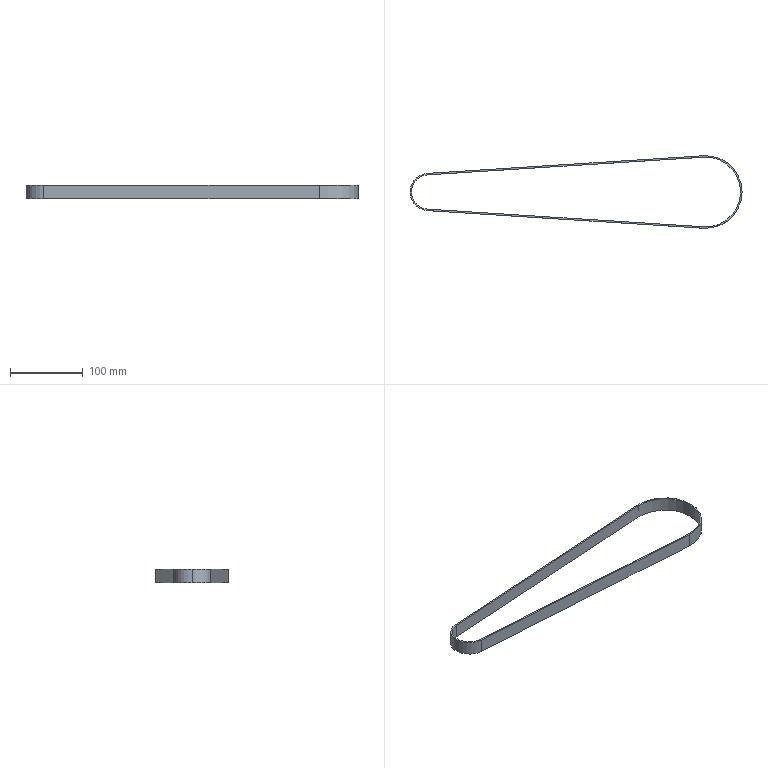Part | STEP file | Timing belt_3 | 1 solid | 12 faces | box 455.684 x 99.713 x 19.05 mm | volume 38426 mm3 | cylinder 6 | plane 6 | commonest cylinder face diameters 47.139 x2 51.203 x2 95.649 x1 99.713 x1
STEP:
#1=CARTESIAN_POINT('',(0.,0.,0.));
#2=DIRECTION('',(0.,0.,1.));
#3=DIRECTION('',(1.,0.,0.));
#4=AXIS2_PLACEMENT_3D('',#1,#2,#3);
#5=CARTESIAN_POINT('',(-101.504,23.521,9.525));
#6=VERTEX_POINT('',#5);
#7=CARTESIAN_POINT('',(-101.504,23.521,-9.525));
#8=VERTEX_POINT('',#7);
#9=CARTESIAN_POINT('',(-101.504,23.521,-9.525));
#10=DIRECTION('',(0.,0.,-1.));
#11=VECTOR('',#10,1.);
#12=LINE('',#9,#11);
#13=CARTESIAN_POINT('',(-100.,0.,0.));
#14=DIRECTION('',(0.,0.,-1.));
#15=DIRECTION('',(-1.,0.,0.));
#16=AXIS2_PLACEMENT_3D('',#13,#14,#15);
#17=CYLINDRICAL_SURFACE('',#16,23.569);
#18=CARTESIAN_POINT('',(1.507,9.525));
#19=DIRECTION('',(0.,1.));
#20=VECTOR('',#19,1.);
#21=LINE('',#18,#20);
#22=(GEOMETRIC_REPRESENTATION_CONTEXT(2)PARAMETRIC_REPRESENTATION_CONTEXT()REPRESENTATION_CONTEXT('',''));
#23=DEFINITIONAL_REPRESENTATION('',(#21),#22);
#24=PCURVE('',#17,#23);
#25=CARTESIAN_POINT('',(-101.504,23.521,-9.525));
#26=DIRECTION('',(0.06379,-0.998,0.));
#27=DIRECTION('',(0.998,0.06379,0.));
#28=AXIS2_PLACEMENT_3D('',#25,#26,#27);
#29=PLANE('',#28);
#30=CARTESIAN_POINT('',(0.,0.));
#31=DIRECTION('',(0.,-1.));
#32=VECTOR('',#31,1.);
#33=LINE('',#30,#32);
#34=(GEOMETRIC_REPRESENTATION_CONTEXT(2)PARAMETRIC_REPRESENTATION_CONTEXT()REPRESENTATION_CONTEXT('',''));
#35=DEFINITIONAL_REPRESENTATION('',(#33),#34);
#36=PCURVE('',#29,#35);
#37=SURFACE_CURVE('',#12,(#24,#36),.PCURVE_S1.);
#38=EDGE_CURVE('',#6,#8,#37,.T.);
#39=ORIENTED_EDGE('',*,*,#38,.T.);
#40=CARTESIAN_POINT('',(-123.569,0.,-9.525));
#41=VERTEX_POINT('',#40);
#42=CARTESIAN_POINT('',(-100.,0.,-9.525));
#43=DIRECTION('',(0.,0.,1.));
#44=DIRECTION('',(-1.,0.,0.));
#45=AXIS2_PLACEMENT_3D('',#42,#43,#44);
#46=CIRCLE('',#45,23.569);
#47=CARTESIAN_POINT('',(6.283,9.525));
#48=DIRECTION('',(-1.,0.));
#49=VECTOR('',#48,1.);
#50=LINE('',#47,#49);
#51=(GEOMETRIC_REPRESENTATION_CONTEXT(2)PARAMETRIC_REPRESENTATION_CONTEXT()REPRESENTATION_CONTEXT('',''));
#52=DEFINITIONAL_REPRESENTATION('',(#50),#51);
#53=PCURVE('',#17,#52);
#54=CARTESIAN_POINT('',(277.11,48.741,-9.525));
#55=DIRECTION('',(0.,0.,-1.));
#56=DIRECTION('',(-1.,0.,0.));
#57=AXIS2_PLACEMENT_3D('',#54,#55,#56);
#58=PLANE('',#57);
#59=CARTESIAN_POINT('',(400.68,-48.741));
#60=CARTESIAN_POINT('',(400.68,-89.565));
#61=CARTESIAN_POINT('',(365.326,-69.153));
#62=CARTESIAN_POINT('',(329.972,-48.741));
#63=CARTESIAN_POINT('',(365.326,-28.329));
#64=CARTESIAN_POINT('',(400.68,-7.918));
#65=CARTESIAN_POINT('',(400.68,-48.741));
#66=(BOUNDED_CURVE()B_SPLINE_CURVE(2,(#59,#60,#61,#62,#63,#64,#65),.UNSPECIFIED.,.T.,.F.)B_SPLINE_CURVE_WITH_KNOTS((1,2,2,2,2,1),(-2.094,0.,2.094,4.189,6.283,8.378),.UNSPECIFIED.)CURVE()GEOMETRIC_REPRESENTATION_ITEM()RATIONAL_B_SPLINE_CURVE((1.,0.5,1.,0.5,1.,0.5,1.))REPRESENTATION_ITEM(''));
#67=(GEOMETRIC_REPRESENTATION_CONTEXT(2)PARAMETRIC_REPRESENTATION_CONTEXT()REPRESENTATION_CONTEXT('',''));
#68=DEFINITIONAL_REPRESENTATION('',(#66),#67);
#69=PCURVE('',#58,#68);
#70=SURFACE_CURVE('',#46,(#53,#69),.PCURVE_S1.);
#71=EDGE_CURVE('',#8,#41,#70,.T.);
#72=ORIENTED_EDGE('',*,*,#71,.T.);
#73=CARTESIAN_POINT('',(-123.569,0.,9.525));
#74=VERTEX_POINT('',#73);
#75=CARTESIAN_POINT('',(-123.569,0.,0.));
#76=DIRECTION('',(0.,0.,-1.));
#77=VECTOR('',#76,1.);
#78=LINE('',#75,#77);
#79=CARTESIAN_POINT('',(0.,0.));
#80=DIRECTION('',(0.,1.));
#81=VECTOR('',#80,1.);
#82=LINE('',#79,#81);
#83=(GEOMETRIC_REPRESENTATION_CONTEXT(2)PARAMETRIC_REPRESENTATION_CONTEXT()REPRESENTATION_CONTEXT('',''));
#84=DEFINITIONAL_REPRESENTATION('',(#82),#83);
#85=PCURVE('',#17,#84);
#86=CARTESIAN_POINT('',(-100.,0.,0.));
#87=DIRECTION('',(0.,0.,-1.));
#88=DIRECTION('',(-1.,0.,0.));
#89=AXIS2_PLACEMENT_3D('',#86,#87,#88);
#90=CYLINDRICAL_SURFACE('',#89,23.569);
#91=CARTESIAN_POINT('',(6.283,0.));
#92=DIRECTION('',(0.,1.));
#93=VECTOR('',#92,1.);
#94=LINE('',#91,#93);
#95=(GEOMETRIC_REPRESENTATION_CONTEXT(2)PARAMETRIC_REPRESENTATION_CONTEXT()REPRESENTATION_CONTEXT('',''));
#96=DEFINITIONAL_REPRESENTATION('',(#94),#95);
#97=PCURVE('',#90,#96);
#98=SURFACE_CURVE('',#78,(#85,#97),.PCURVE_S1.);
#99=EDGE_CURVE('',#74,#41,#98,.T.);
#100=ORIENTED_EDGE('',*,*,#99,.F.);
#101=CARTESIAN_POINT('',(-100.,0.,9.525));
#102=DIRECTION('',(0.,0.,-1.));
#103=DIRECTION('',(-1.,0.,0.));
#104=AXIS2_PLACEMENT_3D('',#101,#102,#103);
#105=CIRCLE('',#104,23.569);
#106=CARTESIAN_POINT('',(0.,-9.525));
#107=DIRECTION('',(1.,0.));
#108=VECTOR('',#107,1.);
#109=LINE('',#106,#108);
#110=(GEOMETRIC_REPRESENTATION_CONTEXT(2)PARAMETRIC_REPRESENTATION_CONTEXT()REPRESENTATION_CONTEXT('',''));
#111=DEFINITIONAL_REPRESENTATION('',(#109),#110);
#112=PCURVE('',#17,#111);
#113=CARTESIAN_POINT('',(277.11,48.741,9.525));
#114=DIRECTION('',(0.,0.,1.));
#115=DIRECTION('',(1.,0.,0.));
#116=AXIS2_PLACEMENT_3D('',#113,#114,#115);
#117=PLANE('',#116);
#118=CARTESIAN_POINT('',(-400.68,-48.741));
#119=CARTESIAN_POINT('',(-400.68,-7.918));
#120=CARTESIAN_POINT('',(-365.326,-28.329));
#121=CARTESIAN_POINT('',(-329.972,-48.741));
#122=CARTESIAN_POINT('',(-365.326,-69.153));
#123=CARTESIAN_POINT('',(-400.68,-89.565));
#124=CARTESIAN_POINT('',(-400.68,-48.741));
#125=(BOUNDED_CURVE()B_SPLINE_CURVE(2,(#118,#119,#120,#121,#122,#123,#124),.UNSPECIFIED.,.T.,.F.)B_SPLINE_CURVE_WITH_KNOTS((1,2,2,2,2,1),(-2.094,0.,2.094,4.189,6.283,8.378),.UNSPECIFIED.)CURVE()GEOMETRIC_REPRESENTATION_ITEM()RATIONAL_B_SPLINE_CURVE((1.,0.5,1.,0.5,1.,0.5,1.))REPRESENTATION_ITEM(''));
#126=(GEOMETRIC_REPRESENTATION_CONTEXT(2)PARAMETRIC_REPRESENTATION_CONTEXT()REPRESENTATION_CONTEXT('',''));
#127=DEFINITIONAL_REPRESENTATION('',(#125),#126);
#128=PCURVE('',#117,#127);
#129=SURFACE_CURVE('',#105,(#112,#128),.PCURVE_S1.);
#130=EDGE_CURVE('',#74,#6,#129,.T.);
#131=ORIENTED_EDGE('',*,*,#130,.T.);
#132=EDGE_LOOP('',(#39,#72,#100,#131));
#133=FACE_BOUND('',#132,.F.);
#134=ADVANCED_FACE('',(#133),#17,.F.);
#135=CARTESIAN_POINT('',(-125.601,0.,9.525));
#136=VERTEX_POINT('',#135);
#137=CARTESIAN_POINT('',(-101.633,-25.549,9.525));
#138=VERTEX_POINT('',#137);
#139=CARTESIAN_POINT('',(-100.,0.,9.525));
#140=DIRECTION('',(0.,0.,1.));
#141=DIRECTION('',(-1.,0.,0.));
#142=AXIS2_PLACEMENT_3D('',#139,#140,#141);
#143=CIRCLE('',#142,25.601);
#144=CARTESIAN_POINT('',(-100.,0.,0.));
#145=DIRECTION('',(0.,0.,-1.));
#146=DIRECTION('',(-1.,0.,0.));
#147=AXIS2_PLACEMENT_3D('',#144,#145,#146);
#148=CYLINDRICAL_SURFACE('',#147,25.601);
#149=CARTESIAN_POINT('',(6.283,-9.525));
#150=DIRECTION('',(-1.,0.));
#151=VECTOR('',#150,1.);
#152=LINE('',#149,#151);
#153=(GEOMETRIC_REPRESENTATION_CONTEXT(2)PARAMETRIC_REPRESENTATION_CONTEXT()REPRESENTATION_CONTEXT('',''));
#154=DEFINITIONAL_REPRESENTATION('',(#152),#153);
#155=PCURVE('',#148,#154);
#156=CARTESIAN_POINT('',(-377.11,-48.741));
#157=DIRECTION('',(-1.,0.));
#158=AXIS2_PLACEMENT_2D('',#156,#157);
#159=CIRCLE('',#158,25.601);
#160=(GEOMETRIC_REPRESENTATION_CONTEXT(2)PARAMETRIC_REPRESENTATION_CONTEXT()REPRESENTATION_CONTEXT('',''));
#161=DEFINITIONAL_REPRESENTATION('',(#159),#160);
#162=PCURVE('',#117,#161);
#163=SURFACE_CURVE('',#143,(#155,#162),.PCURVE_S1.);
#164=EDGE_CURVE('',#136,#138,#163,.T.);
#165=ORIENTED_EDGE('',*,*,#164,.F.);
#166=CARTESIAN_POINT('',(-125.601,0.,-9.525));
#167=VERTEX_POINT('',#166);
#168=CARTESIAN_POINT('',(-125.601,0.,0.));
#169=DIRECTION('',(0.,0.,-1.));
#170=VECTOR('',#169,1.);
#171=LINE('',#168,#170);
#172=CARTESIAN_POINT('',(6.283,0.));
#173=DIRECTION('',(0.,1.));
#174=VECTOR('',#173,1.);
#175=LINE('',#172,#174);
#176=(GEOMETRIC_REPRESENTATION_CONTEXT(2)PARAMETRIC_REPRESENTATION_CONTEXT()REPRESENTATION_CONTEXT('',''));
#177=DEFINITIONAL_REPRESENTATION('',(#175),#176);
#178=PCURVE('',#148,#177);
#179=CARTESIAN_POINT('',(-100.,0.,0.));
#180=DIRECTION('',(0.,0.,-1.));
#181=DIRECTION('',(-1.,0.,0.));
#182=AXIS2_PLACEMENT_3D('',#179,#180,#181);
#183=CYLINDRICAL_SURFACE('',#182,25.601);
#184=CARTESIAN_POINT('',(0.,0.));
#185=DIRECTION('',(0.,1.));
#186=VECTOR('',#185,1.);
#187=LINE('',#184,#186);
#188=(GEOMETRIC_REPRESENTATION_CONTEXT(2)PARAMETRIC_REPRESENTATION_CONTEXT()REPRESENTATION_CONTEXT('',''));
#189=DEFINITIONAL_REPRESENTATION('',(#187),#188);
#190=PCURVE('',#183,#189);
#191=SURFACE_CURVE('',#171,(#178,#190),.PCURVE_S1.);
#192=EDGE_CURVE('',#136,#167,#191,.T.);
#193=ORIENTED_EDGE('',*,*,#192,.T.);
#194=CARTESIAN_POINT('',(-101.633,-25.549,-9.525));
#195=VERTEX_POINT('',#194);
#196=CARTESIAN_POINT('',(-100.,0.,-9.525));
#197=DIRECTION('',(0.,0.,-1.));
#198=DIRECTION('',(-1.,0.,0.));
#199=AXIS2_PLACEMENT_3D('',#196,#197,#198);
#200=CIRCLE('',#199,25.601);
#201=CARTESIAN_POINT('',(0.,9.525));
#202=DIRECTION('',(1.,0.));
#203=VECTOR('',#202,1.);
#204=LINE('',#201,#203);
#205=(GEOMETRIC_REPRESENTATION_CONTEXT(2)PARAMETRIC_REPRESENTATION_CONTEXT()REPRESENTATION_CONTEXT('',''));
#206=DEFINITIONAL_REPRESENTATION('',(#204),#205);
#207=PCURVE('',#148,#206);
#208=CARTESIAN_POINT('',(377.11,-48.741));
#209=DIRECTION('',(1.,0.));
#210=AXIS2_PLACEMENT_2D('',#208,#209);
#211=CIRCLE('',#210,25.601);
#212=(GEOMETRIC_REPRESENTATION_CONTEXT(2)PARAMETRIC_REPRESENTATION_CONTEXT()REPRESENTATION_CONTEXT('',''));
#213=DEFINITIONAL_REPRESENTATION('',(#211),#212);
#214=PCURVE('',#58,#213);
#215=SURFACE_CURVE('',#200,(#207,#214),.PCURVE_S1.);
#216=EDGE_CURVE('',#195,#167,#215,.T.);
#217=ORIENTED_EDGE('',*,*,#216,.F.);
#218=CARTESIAN_POINT('',(-101.633,-25.549,0.));
#219=DIRECTION('',(0.,0.,1.));
#220=VECTOR('',#219,1.);
#221=LINE('',#218,#220);
#222=CARTESIAN_POINT('',(4.776,0.));
#223=DIRECTION('',(0.,-1.));
#224=VECTOR('',#223,1.);
#225=LINE('',#222,#224);
#226=(GEOMETRIC_REPRESENTATION_CONTEXT(2)PARAMETRIC_REPRESENTATION_CONTEXT()REPRESENTATION_CONTEXT('',''));
#227=DEFINITIONAL_REPRESENTATION('',(#225),#226);
#228=PCURVE('',#148,#227);
#229=CARTESIAN_POINT('',(277.046,-49.755,9.525));
#230=DIRECTION('',(-0.06379,-0.998,0.));
#231=DIRECTION('',(0.998,-0.06379,0.));
#232=AXIS2_PLACEMENT_3D('',#229,#230,#231);
#233=PLANE('',#232);
#234=CARTESIAN_POINT('',(-379.452,-9.525));
#235=DIRECTION('',(0.,1.));
#236=VECTOR('',#235,1.);
#237=LINE('',#234,#236);
#238=(GEOMETRIC_REPRESENTATION_CONTEXT(2)PARAMETRIC_REPRESENTATION_CONTEXT()REPRESENTATION_CONTEXT('',''));
#239=DEFINITIONAL_REPRESENTATION('',(#237),#238);
#240=PCURVE('',#233,#239);
#241=SURFACE_CURVE('',#221,(#228,#240),.PCURVE_S1.);
#242=EDGE_CURVE('',#195,#138,#241,.T.);
#243=ORIENTED_EDGE('',*,*,#242,.T.);
#244=EDGE_LOOP('',(#165,#193,#217,#243));
#245=FACE_BOUND('',#244,.T.);
#246=ADVANCED_FACE('',(#245),#148,.T.);
#247=ORIENTED_EDGE('',*,*,#38,.T.);
#248=CARTESIAN_POINT('',(277.175,47.727,-9.525));
#249=VERTEX_POINT('',#248);
#250=CARTESIAN_POINT('',(-101.504,23.521,-9.525));
#251=DIRECTION('',(0.998,0.06379,0.));
#252=VECTOR('',#251,1.);
#253=LINE('',#250,#252);
#254=CARTESIAN_POINT('',(0.,0.));
#255=DIRECTION('',(1.,0.));
#256=VECTOR('',#255,1.);
#257=LINE('',#254,#256);
#258=(GEOMETRIC_REPRESENTATION_CONTEXT(2)PARAMETRIC_REPRESENTATION_CONTEXT()REPRESENTATION_CONTEXT('',''));
#259=DEFINITIONAL_REPRESENTATION('',(#257),#258);
#260=PCURVE('',#29,#259);
#261=CARTESIAN_POINT('',(378.614,-25.22));
#262=DIRECTION('',(-0.998,0.06379));
#263=VECTOR('',#262,1.);
#264=LINE('',#261,#263);
#265=(GEOMETRIC_REPRESENTATION_CONTEXT(2)PARAMETRIC_REPRESENTATION_CONTEXT()REPRESENTATION_CONTEXT('',''));
#266=DEFINITIONAL_REPRESENTATION('',(#264),#265);
#267=PCURVE('',#58,#266);
#268=SURFACE_CURVE('',#253,(#260,#267),.PCURVE_S1.);
#269=EDGE_CURVE('',#8,#249,#268,.T.);
#270=ORIENTED_EDGE('',*,*,#269,.T.);
#271=CARTESIAN_POINT('',(277.175,47.727,9.525));
#272=VERTEX_POINT('',#271);
#273=CARTESIAN_POINT('',(277.175,47.727,-9.525));
#274=DIRECTION('',(0.,0.,1.));
#275=VECTOR('',#274,1.);
#276=LINE('',#273,#275);
#277=CARTESIAN_POINT('',(379.452,0.));
#278=DIRECTION('',(0.,1.));
#279=VECTOR('',#278,1.);
#280=LINE('',#277,#279);
#281=(GEOMETRIC_REPRESENTATION_CONTEXT(2)PARAMETRIC_REPRESENTATION_CONTEXT()REPRESENTATION_CONTEXT('',''));
#282=DEFINITIONAL_REPRESENTATION('',(#280),#281);
#283=PCURVE('',#29,#282);
#284=CARTESIAN_POINT('',(280.226,0.,0.));
#285=DIRECTION('',(0.,0.,-1.));
#286=DIRECTION('',(-1.,0.,0.));
#287=AXIS2_PLACEMENT_3D('',#284,#285,#286);
#288=CYLINDRICAL_SURFACE('',#287,47.825);
#289=CARTESIAN_POINT('',(1.507,9.525));
#290=DIRECTION('',(0.,-1.));
#291=VECTOR('',#290,1.);
#292=LINE('',#289,#291);
#293=(GEOMETRIC_REPRESENTATION_CONTEXT(2)PARAMETRIC_REPRESENTATION_CONTEXT()REPRESENTATION_CONTEXT('',''));
#294=DEFINITIONAL_REPRESENTATION('',(#292),#293);
#295=PCURVE('',#288,#294);
#296=SURFACE_CURVE('',#276,(#283,#295),.PCURVE_S1.);
#297=EDGE_CURVE('',#249,#272,#296,.T.);
#298=ORIENTED_EDGE('',*,*,#297,.T.);
#299=CARTESIAN_POINT('',(-101.504,23.521,9.525));
#300=DIRECTION('',(-0.998,-0.06379,0.));
#301=VECTOR('',#300,1.);
#302=LINE('',#299,#301);
#303=CARTESIAN_POINT('',(0.,19.05));
#304=DIRECTION('',(-1.,0.));
#305=VECTOR('',#304,1.);
#306=LINE('',#303,#305);
#307=(GEOMETRIC_REPRESENTATION_CONTEXT(2)PARAMETRIC_REPRESENTATION_CONTEXT()REPRESENTATION_CONTEXT('',''));
#308=DEFINITIONAL_REPRESENTATION('',(#306),#307);
#309=PCURVE('',#29,#308);
#310=CARTESIAN_POINT('',(-378.614,-25.22));
#311=DIRECTION('',(-0.998,-0.06379));
#312=VECTOR('',#311,1.);
#313=LINE('',#310,#312);
#314=(GEOMETRIC_REPRESENTATION_CONTEXT(2)PARAMETRIC_REPRESENTATION_CONTEXT()REPRESENTATION_CONTEXT('',''));
#315=DEFINITIONAL_REPRESENTATION('',(#313),#314);
#316=PCURVE('',#117,#315);
#317=SURFACE_CURVE('',#302,(#309,#316),.PCURVE_S1.);
#318=EDGE_CURVE('',#272,#6,#317,.T.);
#319=ORIENTED_EDGE('',*,*,#318,.T.);
#320=EDGE_LOOP('',(#247,#270,#298,#319));
#321=FACE_BOUND('',#320,.T.);
#322=ADVANCED_FACE('',(#321),#29,.T.);
#323=CARTESIAN_POINT('',(-101.504,-23.521,-9.525));
#324=VERTEX_POINT('',#323);
#325=CARTESIAN_POINT('',(277.175,-47.727,-9.525));
#326=VERTEX_POINT('',#325);
#327=CARTESIAN_POINT('',(-101.504,-23.521,-9.525));
#328=DIRECTION('',(0.998,-0.06379,0.));
#329=VECTOR('',#328,1.);
#330=LINE('',#327,#329);
#331=CARTESIAN_POINT('',(378.614,-72.263));
#332=DIRECTION('',(-0.998,-0.06379));
#333=VECTOR('',#332,1.);
#334=LINE('',#331,#333);
#335=(GEOMETRIC_REPRESENTATION_CONTEXT(2)PARAMETRIC_REPRESENTATION_CONTEXT()REPRESENTATION_CONTEXT('',''));
#336=DEFINITIONAL_REPRESENTATION('',(#334),#335);
#337=PCURVE('',#58,#336);
#338=CARTESIAN_POINT('',(277.175,-47.727,-9.525));
#339=DIRECTION('',(0.06379,0.998,0.));
#340=DIRECTION('',(-0.998,0.06379,0.));
#341=AXIS2_PLACEMENT_3D('',#338,#339,#340);
#342=PLANE('',#341);
#343=CARTESIAN_POINT('',(379.452,0.));
#344=DIRECTION('',(-1.,0.));
#345=VECTOR('',#344,1.);
#346=LINE('',#343,#345);
#347=(GEOMETRIC_REPRESENTATION_CONTEXT(2)PARAMETRIC_REPRESENTATION_CONTEXT()REPRESENTATION_CONTEXT('',''));
#348=DEFINITIONAL_REPRESENTATION('',(#346),#347);
#349=PCURVE('',#342,#348);
#350=SURFACE_CURVE('',#330,(#337,#349),.PCURVE_S1.);
#351=EDGE_CURVE('',#324,#326,#350,.T.);
#352=ORIENTED_EDGE('',*,*,#351,.T.);
#353=CARTESIAN_POINT('',(280.226,0.,-9.525));
#354=DIRECTION('',(0.,0.,1.));
#355=DIRECTION('',(-1.,0.,0.));
#356=AXIS2_PLACEMENT_3D('',#353,#354,#355);
#357=CIRCLE('',#356,47.825);
#358=CARTESIAN_POINT('',(44.709,-48.741));
#359=CARTESIAN_POINT('',(44.709,-131.576));
#360=CARTESIAN_POINT('',(-27.028,-90.158));
#361=CARTESIAN_POINT('',(-98.765,-48.741));
#362=CARTESIAN_POINT('',(-27.028,-7.324));
#363=CARTESIAN_POINT('',(44.709,34.094));
#364=CARTESIAN_POINT('',(44.709,-48.741));
#365=(BOUNDED_CURVE()B_SPLINE_CURVE(2,(#358,#359,#360,#361,#362,#363,#364),.UNSPECIFIED.,.T.,.F.)B_SPLINE_CURVE_WITH_KNOTS((1,2,2,2,2,1),(-2.094,0.,2.094,4.189,6.283,8.378),.UNSPECIFIED.)CURVE()GEOMETRIC_REPRESENTATION_ITEM()RATIONAL_B_SPLINE_CURVE((1.,0.5,1.,0.5,1.,0.5,1.))REPRESENTATION_ITEM(''));
#366=(GEOMETRIC_REPRESENTATION_CONTEXT(2)PARAMETRIC_REPRESENTATION_CONTEXT()REPRESENTATION_CONTEXT('',''));
#367=DEFINITIONAL_REPRESENTATION('',(#365),#366);
#368=PCURVE('',#58,#367);
#369=CARTESIAN_POINT('',(6.283,9.525));
#370=DIRECTION('',(-1.,0.));
#371=VECTOR('',#370,1.);
#372=LINE('',#369,#371);
#373=(GEOMETRIC_REPRESENTATION_CONTEXT(2)PARAMETRIC_REPRESENTATION_CONTEXT()REPRESENTATION_CONTEXT('',''));
#374=DEFINITIONAL_REPRESENTATION('',(#372),#373);
#375=PCURVE('',#288,#374);
#376=SURFACE_CURVE('',#357,(#368,#375),.PCURVE_S1.);
#377=EDGE_CURVE('',#326,#249,#376,.T.);
#378=ORIENTED_EDGE('',*,*,#377,.T.);
#379=ORIENTED_EDGE('',*,*,#269,.F.);
#380=ORIENTED_EDGE('',*,*,#71,.T.);
#381=CARTESIAN_POINT('',(-100.,0.,-9.525));
#382=DIRECTION('',(0.,0.,1.));
#383=DIRECTION('',(-1.,0.,0.));
#384=AXIS2_PLACEMENT_3D('',#381,#382,#383);
#385=CIRCLE('',#384,23.569);
#386=CARTESIAN_POINT('',(400.68,-48.741));
#387=CARTESIAN_POINT('',(400.68,-89.565));
#388=CARTESIAN_POINT('',(365.326,-69.153));
#389=CARTESIAN_POINT('',(329.972,-48.741));
#390=CARTESIAN_POINT('',(365.326,-28.329));
#391=CARTESIAN_POINT('',(400.68,-7.918));
#392=CARTESIAN_POINT('',(400.68,-48.741));
#393=(BOUNDED_CURVE()B_SPLINE_CURVE(2,(#386,#387,#388,#389,#390,#391,#392),.UNSPECIFIED.,.T.,.F.)B_SPLINE_CURVE_WITH_KNOTS((1,2,2,2,2,1),(-2.094,0.,2.094,4.189,6.283,8.378),.UNSPECIFIED.)CURVE()GEOMETRIC_REPRESENTATION_ITEM()RATIONAL_B_SPLINE_CURVE((1.,0.5,1.,0.5,1.,0.5,1.))REPRESENTATION_ITEM(''));
#394=(GEOMETRIC_REPRESENTATION_CONTEXT(2)PARAMETRIC_REPRESENTATION_CONTEXT()REPRESENTATION_CONTEXT('',''));
#395=DEFINITIONAL_REPRESENTATION('',(#393),#394);
#396=PCURVE('',#58,#395);
#397=CARTESIAN_POINT('',(6.283,9.525));
#398=DIRECTION('',(-1.,0.));
#399=VECTOR('',#398,1.);
#400=LINE('',#397,#399);
#401=(GEOMETRIC_REPRESENTATION_CONTEXT(2)PARAMETRIC_REPRESENTATION_CONTEXT()REPRESENTATION_CONTEXT('',''));
#402=DEFINITIONAL_REPRESENTATION('',(#400),#401);
#403=PCURVE('',#90,#402);
#404=SURFACE_CURVE('',#385,(#396,#403),.PCURVE_S1.);
#405=EDGE_CURVE('',#41,#324,#404,.T.);
#406=ORIENTED_EDGE('',*,*,#405,.T.);
#407=EDGE_LOOP('',(#352,#378,#379,#380,#406));
#408=FACE_BOUND('',#407,.T.);
#409=ORIENTED_EDGE('',*,*,#216,.T.);
#410=CARTESIAN_POINT('',(-101.633,25.549,-9.525));
#411=VERTEX_POINT('',#410);
#412=CARTESIAN_POINT('',(-100.,0.,-9.525));
#413=DIRECTION('',(0.,0.,-1.));
#414=DIRECTION('',(-1.,0.,0.));
#415=AXIS2_PLACEMENT_3D('',#412,#413,#414);
#416=CIRCLE('',#415,25.601);
#417=CARTESIAN_POINT('',(377.11,-48.741));
#418=DIRECTION('',(1.,0.));
#419=AXIS2_PLACEMENT_2D('',#417,#418);
#420=CIRCLE('',#419,25.601);
#421=(GEOMETRIC_REPRESENTATION_CONTEXT(2)PARAMETRIC_REPRESENTATION_CONTEXT()REPRESENTATION_CONTEXT('',''));
#422=DEFINITIONAL_REPRESENTATION('',(#420),#421);
#423=PCURVE('',#58,#422);
#424=CARTESIAN_POINT('',(0.,9.525));
#425=DIRECTION('',(1.,0.));
#426=VECTOR('',#425,1.);
#427=LINE('',#424,#426);
#428=(GEOMETRIC_REPRESENTATION_CONTEXT(2)PARAMETRIC_REPRESENTATION_CONTEXT()REPRESENTATION_CONTEXT('',''));
#429=DEFINITIONAL_REPRESENTATION('',(#427),#428);
#430=PCURVE('',#183,#429);
#431=SURFACE_CURVE('',#416,(#423,#430),.PCURVE_S1.);
#432=EDGE_CURVE('',#167,#411,#431,.T.);
#433=ORIENTED_EDGE('',*,*,#432,.T.);
#434=CARTESIAN_POINT('',(277.046,49.755,-9.525));
#435=VERTEX_POINT('',#434);
#436=CARTESIAN_POINT('',(-101.633,25.549,-9.525));
#437=DIRECTION('',(0.998,0.06379,0.));
#438=VECTOR('',#437,1.);
#439=LINE('',#436,#438);
#440=CARTESIAN_POINT('',(378.744,-23.192));
#441=DIRECTION('',(-0.998,0.06379));
#442=VECTOR('',#441,1.);
#443=LINE('',#440,#442);
#444=(GEOMETRIC_REPRESENTATION_CONTEXT(2)PARAMETRIC_REPRESENTATION_CONTEXT()REPRESENTATION_CONTEXT('',''));
#445=DEFINITIONAL_REPRESENTATION('',(#443),#444);
#446=PCURVE('',#58,#445);
#447=CARTESIAN_POINT('',(-101.633,25.549,9.525));
#448=DIRECTION('',(-0.06379,0.998,0.));
#449=DIRECTION('',(-0.998,-0.06379,0.));
#450=AXIS2_PLACEMENT_3D('',#447,#448,#449);
#451=PLANE('',#450);
#452=CARTESIAN_POINT('',(0.,-19.05));
#453=DIRECTION('',(-1.,0.));
#454=VECTOR('',#453,1.);
#455=LINE('',#452,#454);
#456=(GEOMETRIC_REPRESENTATION_CONTEXT(2)PARAMETRIC_REPRESENTATION_CONTEXT()REPRESENTATION_CONTEXT('',''));
#457=DEFINITIONAL_REPRESENTATION('',(#455),#456);
#458=PCURVE('',#451,#457);
#459=SURFACE_CURVE('',#439,(#446,#458),.PCURVE_S1.);
#460=EDGE_CURVE('',#411,#435,#459,.T.);
#461=ORIENTED_EDGE('',*,*,#460,.T.);
#462=CARTESIAN_POINT('',(277.046,-49.755,-9.525));
#463=VERTEX_POINT('',#462);
#464=CARTESIAN_POINT('',(280.226,0.,-9.525));
#465=DIRECTION('',(0.,0.,-1.));
#466=DIRECTION('',(-1.,0.,0.));
#467=AXIS2_PLACEMENT_3D('',#464,#465,#466);
#468=CIRCLE('',#467,49.857);
#469=CARTESIAN_POINT('',(-3.116,-48.741));
#470=DIRECTION('',(1.,0.));
#471=AXIS2_PLACEMENT_2D('',#469,#470);
#472=CIRCLE('',#471,49.857);
#473=(GEOMETRIC_REPRESENTATION_CONTEXT(2)PARAMETRIC_REPRESENTATION_CONTEXT()REPRESENTATION_CONTEXT('',''));
#474=DEFINITIONAL_REPRESENTATION('',(#472),#473);
#475=PCURVE('',#58,#474);
#476=CARTESIAN_POINT('',(280.226,0.,0.));
#477=DIRECTION('',(0.,0.,-1.));
#478=DIRECTION('',(-1.,0.,0.));
#479=AXIS2_PLACEMENT_3D('',#476,#477,#478);
#480=CYLINDRICAL_SURFACE('',#479,49.857);
#481=CARTESIAN_POINT('',(0.,9.525));
#482=DIRECTION('',(1.,0.));
#483=VECTOR('',#482,1.);
#484=LINE('',#481,#483);
#485=(GEOMETRIC_REPRESENTATION_CONTEXT(2)PARAMETRIC_REPRESENTATION_CONTEXT()REPRESENTATION_CONTEXT('',''));
#486=DEFINITIONAL_REPRESENTATION('',(#484),#485);
#487=PCURVE('',#480,#486);
#488=SURFACE_CURVE('',#468,(#475,#487),.PCURVE_S1.);
#489=EDGE_CURVE('',#435,#463,#488,.T.);
#490=ORIENTED_EDGE('',*,*,#489,.T.);
#491=CARTESIAN_POINT('',(277.046,-49.755,-9.525));
#492=DIRECTION('',(-0.998,0.06379,0.));
#493=VECTOR('',#492,1.);
#494=LINE('',#491,#493);
#495=CARTESIAN_POINT('',(0.06481,-98.496));
#496=DIRECTION('',(0.998,0.06379));
#497=VECTOR('',#496,1.);
#498=LINE('',#495,#497);
#499=(GEOMETRIC_REPRESENTATION_CONTEXT(2)PARAMETRIC_REPRESENTATION_CONTEXT()REPRESENTATION_CONTEXT('',''));
#500=DEFINITIONAL_REPRESENTATION('',(#498),#499);
#501=PCURVE('',#58,#500);
#502=CARTESIAN_POINT('',(0.,-19.05));
#503=DIRECTION('',(-1.,0.));
#504=VECTOR('',#503,1.);
#505=LINE('',#502,#504);
#506=(GEOMETRIC_REPRESENTATION_CONTEXT(2)PARAMETRIC_REPRESENTATION_CONTEXT()REPRESENTATION_CONTEXT('',''));
#507=DEFINITIONAL_REPRESENTATION('',(#505),#506);
#508=PCURVE('',#233,#507);
#509=SURFACE_CURVE('',#494,(#501,#508),.PCURVE_S1.);
#510=EDGE_CURVE('',#463,#195,#509,.T.);
#511=ORIENTED_EDGE('',*,*,#510,.T.);
#512=EDGE_LOOP('',(#409,#433,#461,#490,#511));
#513=FACE_BOUND('',#512,.T.);
#514=ADVANCED_FACE('',(#408,#513),#58,.T.);
#515=ORIENTED_EDGE('',*,*,#405,.T.);
#516=CARTESIAN_POINT('',(-101.504,-23.521,9.525));
#517=VERTEX_POINT('',#516);
#518=CARTESIAN_POINT('',(-101.504,-23.521,0.));
#519=DIRECTION('',(0.,0.,1.));
#520=VECTOR('',#519,1.);
#521=LINE('',#518,#520);
#522=CARTESIAN_POINT('',(4.776,0.));
#523=DIRECTION('',(0.,-1.));
#524=VECTOR('',#523,1.);
#525=LINE('',#522,#524);
#526=(GEOMETRIC_REPRESENTATION_CONTEXT(2)PARAMETRIC_REPRESENTATION_CONTEXT()REPRESENTATION_CONTEXT('',''));
#527=DEFINITIONAL_REPRESENTATION('',(#525),#526);
#528=PCURVE('',#90,#527);
#529=CARTESIAN_POINT('',(379.452,9.525));
#530=DIRECTION('',(0.,1.));
#531=VECTOR('',#530,1.);
#532=LINE('',#529,#531);
#533=(GEOMETRIC_REPRESENTATION_CONTEXT(2)PARAMETRIC_REPRESENTATION_CONTEXT()REPRESENTATION_CONTEXT('',''));
#534=DEFINITIONAL_REPRESENTATION('',(#532),#533);
#535=PCURVE('',#342,#534);
#536=SURFACE_CURVE('',#521,(#528,#535),.PCURVE_S1.);
#537=EDGE_CURVE('',#324,#517,#536,.T.);
#538=ORIENTED_EDGE('',*,*,#537,.T.);
#539=CARTESIAN_POINT('',(-100.,0.,9.525));
#540=DIRECTION('',(0.,0.,-1.));
#541=DIRECTION('',(-1.,0.,0.));
#542=AXIS2_PLACEMENT_3D('',#539,#540,#541);
#543=CIRCLE('',#542,23.569);
#544=CARTESIAN_POINT('',(0.,-9.525));
#545=DIRECTION('',(1.,0.));
#546=VECTOR('',#545,1.);
#547=LINE('',#544,#546);
#548=(GEOMETRIC_REPRESENTATION_CONTEXT(2)PARAMETRIC_REPRESENTATION_CONTEXT()REPRESENTATION_CONTEXT('',''));
#549=DEFINITIONAL_REPRESENTATION('',(#547),#548);
#550=PCURVE('',#90,#549);
#551=CARTESIAN_POINT('',(-400.68,-48.741));
#552=CARTESIAN_POINT('',(-400.68,-7.918));
#553=CARTESIAN_POINT('',(-365.326,-28.329));
#554=CARTESIAN_POINT('',(-329.972,-48.741));
#555=CARTESIAN_POINT('',(-365.326,-69.153));
#556=CARTESIAN_POINT('',(-400.68,-89.565));
#557=CARTESIAN_POINT('',(-400.68,-48.741));
#558=(BOUNDED_CURVE()B_SPLINE_CURVE(2,(#551,#552,#553,#554,#555,#556,#557),.UNSPECIFIED.,.T.,.F.)B_SPLINE_CURVE_WITH_KNOTS((1,2,2,2,2,1),(-2.094,0.,2.094,4.189,6.283,8.378),.UNSPECIFIED.)CURVE()GEOMETRIC_REPRESENTATION_ITEM()RATIONAL_B_SPLINE_CURVE((1.,0.5,1.,0.5,1.,0.5,1.))REPRESENTATION_ITEM(''));
#559=(GEOMETRIC_REPRESENTATION_CONTEXT(2)PARAMETRIC_REPRESENTATION_CONTEXT()REPRESENTATION_CONTEXT('',''));
#560=DEFINITIONAL_REPRESENTATION('',(#558),#559);
#561=PCURVE('',#117,#560);
#562=SURFACE_CURVE('',#543,(#550,#561),.PCURVE_S1.);
#563=EDGE_CURVE('',#517,#74,#562,.T.);
#564=ORIENTED_EDGE('',*,*,#563,.T.);
#565=ORIENTED_EDGE('',*,*,#99,.T.);
#566=EDGE_LOOP('',(#515,#538,#564,#565));
#567=FACE_BOUND('',#566,.F.);
#568=ADVANCED_FACE('',(#567),#90,.F.);
#569=ORIENTED_EDGE('',*,*,#563,.T.);
#570=ORIENTED_EDGE('',*,*,#130,.T.);
#571=ORIENTED_EDGE('',*,*,#318,.F.);
#572=CARTESIAN_POINT('',(277.175,-47.727,9.525));
#573=VERTEX_POINT('',#572);
#574=CARTESIAN_POINT('',(280.226,0.,9.525));
#575=DIRECTION('',(0.,0.,-1.));
#576=DIRECTION('',(-1.,0.,0.));
#577=AXIS2_PLACEMENT_3D('',#574,#575,#576);
#578=CIRCLE('',#577,47.825);
#579=CARTESIAN_POINT('',(-44.709,-48.741));
#580=CARTESIAN_POINT('',(-44.709,34.094));
#581=CARTESIAN_POINT('',(27.028,-7.324));
#582=CARTESIAN_POINT('',(98.765,-48.741));
#583=CARTESIAN_POINT('',(27.028,-90.158));
#584=CARTESIAN_POINT('',(-44.709,-131.576));
#585=CARTESIAN_POINT('',(-44.709,-48.741));
#586=(BOUNDED_CURVE()B_SPLINE_CURVE(2,(#579,#580,#581,#582,#583,#584,#585),.UNSPECIFIED.,.T.,.F.)B_SPLINE_CURVE_WITH_KNOTS((1,2,2,2,2,1),(-2.094,0.,2.094,4.189,6.283,8.378),.UNSPECIFIED.)CURVE()GEOMETRIC_REPRESENTATION_ITEM()RATIONAL_B_SPLINE_CURVE((1.,0.5,1.,0.5,1.,0.5,1.))REPRESENTATION_ITEM(''));
#587=(GEOMETRIC_REPRESENTATION_CONTEXT(2)PARAMETRIC_REPRESENTATION_CONTEXT()REPRESENTATION_CONTEXT('',''));
#588=DEFINITIONAL_REPRESENTATION('',(#586),#587);
#589=PCURVE('',#117,#588);
#590=CARTESIAN_POINT('',(0.,-9.525));
#591=DIRECTION('',(1.,0.));
#592=VECTOR('',#591,1.);
#593=LINE('',#590,#592);
#594=(GEOMETRIC_REPRESENTATION_CONTEXT(2)PARAMETRIC_REPRESENTATION_CONTEXT()REPRESENTATION_CONTEXT('',''));
#595=DEFINITIONAL_REPRESENTATION('',(#593),#594);
#596=PCURVE('',#288,#595);
#597=SURFACE_CURVE('',#578,(#589,#596),.PCURVE_S1.);
#598=EDGE_CURVE('',#272,#573,#597,.T.);
#599=ORIENTED_EDGE('',*,*,#598,.T.);
#600=CARTESIAN_POINT('',(277.175,-47.727,9.525));
#601=DIRECTION('',(-0.998,0.06379,0.));
#602=VECTOR('',#601,1.);
#603=LINE('',#600,#602);
#604=CARTESIAN_POINT('',(0.06481,-96.468));
#605=DIRECTION('',(-0.998,0.06379));
#606=VECTOR('',#605,1.);
#607=LINE('',#604,#606);
#608=(GEOMETRIC_REPRESENTATION_CONTEXT(2)PARAMETRIC_REPRESENTATION_CONTEXT()REPRESENTATION_CONTEXT('',''));
#609=DEFINITIONAL_REPRESENTATION('',(#607),#608);
#610=PCURVE('',#117,#609);
#611=CARTESIAN_POINT('',(0.,19.05));
#612=DIRECTION('',(1.,0.));
#613=VECTOR('',#612,1.);
#614=LINE('',#611,#613);
#615=(GEOMETRIC_REPRESENTATION_CONTEXT(2)PARAMETRIC_REPRESENTATION_CONTEXT()REPRESENTATION_CONTEXT('',''));
#616=DEFINITIONAL_REPRESENTATION('',(#614),#615);
#617=PCURVE('',#342,#616);
#618=SURFACE_CURVE('',#603,(#610,#617),.PCURVE_S1.);
#619=EDGE_CURVE('',#573,#517,#618,.T.);
#620=ORIENTED_EDGE('',*,*,#619,.T.);
#621=EDGE_LOOP('',(#569,#570,#571,#599,#620));
#622=FACE_BOUND('',#621,.T.);
#623=CARTESIAN_POINT('',(277.046,-49.755,9.525));
#624=VERTEX_POINT('',#623);
#625=CARTESIAN_POINT('',(-101.633,-25.549,9.525));
#626=DIRECTION('',(0.998,-0.06379,0.));
#627=VECTOR('',#626,1.);
#628=LINE('',#625,#627);
#629=CARTESIAN_POINT('',(-378.744,-74.29));
#630=DIRECTION('',(0.998,-0.06379));
#631=VECTOR('',#630,1.);
#632=LINE('',#629,#631);
#633=(GEOMETRIC_REPRESENTATION_CONTEXT(2)PARAMETRIC_REPRESENTATION_CONTEXT()REPRESENTATION_CONTEXT('',''));
#634=DEFINITIONAL_REPRESENTATION('',(#632),#633);
#635=PCURVE('',#117,#634);
#636=CARTESIAN_POINT('',(-379.452,0.));
#637=DIRECTION('',(1.,0.));
#638=VECTOR('',#637,1.);
#639=LINE('',#636,#638);
#640=(GEOMETRIC_REPRESENTATION_CONTEXT(2)PARAMETRIC_REPRESENTATION_CONTEXT()REPRESENTATION_CONTEXT('',''));
#641=DEFINITIONAL_REPRESENTATION('',(#639),#640);
#642=PCURVE('',#233,#641);
#643=SURFACE_CURVE('',#628,(#635,#642),.PCURVE_S1.);
#644=EDGE_CURVE('',#138,#624,#643,.T.);
#645=ORIENTED_EDGE('',*,*,#644,.T.);
#646=CARTESIAN_POINT('',(277.046,49.755,9.525));
#647=VERTEX_POINT('',#646);
#648=CARTESIAN_POINT('',(280.226,0.,9.525));
#649=DIRECTION('',(0.,0.,1.));
#650=DIRECTION('',(-1.,0.,0.));
#651=AXIS2_PLACEMENT_3D('',#648,#649,#650);
#652=CIRCLE('',#651,49.857);
#653=CARTESIAN_POINT('',(3.116,-48.741));
#654=DIRECTION('',(-1.,0.));
#655=AXIS2_PLACEMENT_2D('',#653,#654);
#656=CIRCLE('',#655,49.857);
#657=(GEOMETRIC_REPRESENTATION_CONTEXT(2)PARAMETRIC_REPRESENTATION_CONTEXT()REPRESENTATION_CONTEXT('',''));
#658=DEFINITIONAL_REPRESENTATION('',(#656),#657);
#659=PCURVE('',#117,#658);
#660=CARTESIAN_POINT('',(6.283,-9.525));
#661=DIRECTION('',(-1.,0.));
#662=VECTOR('',#661,1.);
#663=LINE('',#660,#662);
#664=(GEOMETRIC_REPRESENTATION_CONTEXT(2)PARAMETRIC_REPRESENTATION_CONTEXT()REPRESENTATION_CONTEXT('',''));
#665=DEFINITIONAL_REPRESENTATION('',(#663),#664);
#666=PCURVE('',#480,#665);
#667=SURFACE_CURVE('',#652,(#659,#666),.PCURVE_S1.);
#668=EDGE_CURVE('',#624,#647,#667,.T.);
#669=ORIENTED_EDGE('',*,*,#668,.T.);
#670=CARTESIAN_POINT('',(-101.633,25.549,9.525));
#671=VERTEX_POINT('',#670);
#672=CARTESIAN_POINT('',(277.046,49.755,9.525));
#673=DIRECTION('',(-0.998,-0.06379,0.));
#674=VECTOR('',#673,1.);
#675=LINE('',#672,#674);
#676=CARTESIAN_POINT('',(-0.06481,1.014));
#677=DIRECTION('',(-0.998,-0.06379));
#678=VECTOR('',#677,1.);
#679=LINE('',#676,#678);
#680=(GEOMETRIC_REPRESENTATION_CONTEXT(2)PARAMETRIC_REPRESENTATION_CONTEXT()REPRESENTATION_CONTEXT('',''));
#681=DEFINITIONAL_REPRESENTATION('',(#679),#680);
#682=PCURVE('',#117,#681);
#683=CARTESIAN_POINT('',(-379.452,0.));
#684=DIRECTION('',(1.,0.));
#685=VECTOR('',#684,1.);
#686=LINE('',#683,#685);
#687=(GEOMETRIC_REPRESENTATION_CONTEXT(2)PARAMETRIC_REPRESENTATION_CONTEXT()REPRESENTATION_CONTEXT('',''));
#688=DEFINITIONAL_REPRESENTATION('',(#686),#687);
#689=PCURVE('',#451,#688);
#690=SURFACE_CURVE('',#675,(#682,#689),.PCURVE_S1.);
#691=EDGE_CURVE('',#647,#671,#690,.T.);
#692=ORIENTED_EDGE('',*,*,#691,.T.);
#693=CARTESIAN_POINT('',(-100.,0.,9.525));
#694=DIRECTION('',(0.,0.,1.));
#695=DIRECTION('',(-1.,0.,0.));
#696=AXIS2_PLACEMENT_3D('',#693,#694,#695);
#697=CIRCLE('',#696,25.601);
#698=CARTESIAN_POINT('',(-377.11,-48.741));
#699=DIRECTION('',(-1.,0.));
#700=AXIS2_PLACEMENT_2D('',#698,#699);
#701=CIRCLE('',#700,25.601);
#702=(GEOMETRIC_REPRESENTATION_CONTEXT(2)PARAMETRIC_REPRESENTATION_CONTEXT()REPRESENTATION_CONTEXT('',''));
#703=DEFINITIONAL_REPRESENTATION('',(#701),#702);
#704=PCURVE('',#117,#703);
#705=CARTESIAN_POINT('',(6.283,-9.525));
#706=DIRECTION('',(-1.,0.));
#707=VECTOR('',#706,1.);
#708=LINE('',#705,#707);
#709=(GEOMETRIC_REPRESENTATION_CONTEXT(2)PARAMETRIC_REPRESENTATION_CONTEXT()REPRESENTATION_CONTEXT('',''));
#710=DEFINITIONAL_REPRESENTATION('',(#708),#709);
#711=PCURVE('',#183,#710);
#712=SURFACE_CURVE('',#697,(#704,#711),.PCURVE_S1.);
#713=EDGE_CURVE('',#671,#136,#712,.T.);
#714=ORIENTED_EDGE('',*,*,#713,.T.);
#715=ORIENTED_EDGE('',*,*,#164,.T.);
#716=EDGE_LOOP('',(#645,#669,#692,#714,#715));
#717=FACE_BOUND('',#716,.T.);
#718=ADVANCED_FACE('',(#622,#717),#117,.T.);
#719=CARTESIAN_POINT('',(277.175,-47.727,0.));
#720=DIRECTION('',(0.,0.,-1.));
#721=VECTOR('',#720,1.);
#722=LINE('',#719,#721);
#723=CARTESIAN_POINT('',(4.776,0.));
#724=DIRECTION('',(0.,1.));
#725=VECTOR('',#724,1.);
#726=LINE('',#723,#725);
#727=(GEOMETRIC_REPRESENTATION_CONTEXT(2)PARAMETRIC_REPRESENTATION_CONTEXT()REPRESENTATION_CONTEXT('',''));
#728=DEFINITIONAL_REPRESENTATION('',(#726),#727);
#729=PCURVE('',#288,#728);
#730=CARTESIAN_POINT('',(0.,9.525));
#731=DIRECTION('',(0.,-1.));
#732=VECTOR('',#731,1.);
#733=LINE('',#730,#732);
#734=(GEOMETRIC_REPRESENTATION_CONTEXT(2)PARAMETRIC_REPRESENTATION_CONTEXT()REPRESENTATION_CONTEXT('',''));
#735=DEFINITIONAL_REPRESENTATION('',(#733),#734);
#736=PCURVE('',#342,#735);
#737=SURFACE_CURVE('',#722,(#729,#736),.PCURVE_S1.);
#738=EDGE_CURVE('',#573,#326,#737,.T.);
#739=ORIENTED_EDGE('',*,*,#738,.T.);
#740=ORIENTED_EDGE('',*,*,#377,.T.);
#741=ORIENTED_EDGE('',*,*,#297,.T.);
#742=ORIENTED_EDGE('',*,*,#598,.T.);
#743=EDGE_LOOP('',(#739,#740,#741,#742));
#744=FACE_BOUND('',#743,.F.);
#745=ADVANCED_FACE('',(#744),#288,.F.);
#746=ORIENTED_EDGE('',*,*,#738,.T.);
#747=ORIENTED_EDGE('',*,*,#351,.F.);
#748=ORIENTED_EDGE('',*,*,#537,.T.);
#749=ORIENTED_EDGE('',*,*,#619,.F.);
#750=EDGE_LOOP('',(#746,#747,#748,#749));
#751=FACE_BOUND('',#750,.T.);
#752=ADVANCED_FACE('',(#751),#342,.T.);
#753=CARTESIAN_POINT('',(-101.633,25.549,9.525));
#754=DIRECTION('',(0.,0.,1.));
#755=VECTOR('',#754,1.);
#756=LINE('',#753,#755);
#757=CARTESIAN_POINT('',(0.,0.));
#758=DIRECTION('',(0.,1.));
#759=VECTOR('',#758,1.);
#760=LINE('',#757,#759);
#761=(GEOMETRIC_REPRESENTATION_CONTEXT(2)PARAMETRIC_REPRESENTATION_CONTEXT()REPRESENTATION_CONTEXT('',''));
#762=DEFINITIONAL_REPRESENTATION('',(#760),#761);
#763=PCURVE('',#451,#762);
#764=CARTESIAN_POINT('',(1.507,-9.525));
#765=DIRECTION('',(0.,-1.));
#766=VECTOR('',#765,1.);
#767=LINE('',#764,#766);
#768=(GEOMETRIC_REPRESENTATION_CONTEXT(2)PARAMETRIC_REPRESENTATION_CONTEXT()REPRESENTATION_CONTEXT('',''));
#769=DEFINITIONAL_REPRESENTATION('',(#767),#768);
#770=PCURVE('',#183,#769);
#771=SURFACE_CURVE('',#756,(#763,#770),.PCURVE_S1.);
#772=EDGE_CURVE('',#411,#671,#771,.T.);
#773=ORIENTED_EDGE('',*,*,#772,.T.);
#774=ORIENTED_EDGE('',*,*,#691,.F.);
#775=CARTESIAN_POINT('',(277.046,49.755,9.525));
#776=DIRECTION('',(0.,0.,-1.));
#777=VECTOR('',#776,1.);
#778=LINE('',#775,#777);
#779=CARTESIAN_POINT('',(-379.452,0.));
#780=DIRECTION('',(0.,-1.));
#781=VECTOR('',#780,1.);
#782=LINE('',#779,#781);
#783=(GEOMETRIC_REPRESENTATION_CONTEXT(2)PARAMETRIC_REPRESENTATION_CONTEXT()REPRESENTATION_CONTEXT('',''));
#784=DEFINITIONAL_REPRESENTATION('',(#782),#783);
#785=PCURVE('',#451,#784);
#786=CARTESIAN_POINT('',(1.507,-9.525));
#787=DIRECTION('',(0.,1.));
#788=VECTOR('',#787,1.);
#789=LINE('',#786,#788);
#790=(GEOMETRIC_REPRESENTATION_CONTEXT(2)PARAMETRIC_REPRESENTATION_CONTEXT()REPRESENTATION_CONTEXT('',''));
#791=DEFINITIONAL_REPRESENTATION('',(#789),#790);
#792=PCURVE('',#480,#791);
#793=SURFACE_CURVE('',#778,(#785,#792),.PCURVE_S1.);
#794=EDGE_CURVE('',#647,#435,#793,.T.);
#795=ORIENTED_EDGE('',*,*,#794,.T.);
#796=ORIENTED_EDGE('',*,*,#460,.F.);
#797=EDGE_LOOP('',(#773,#774,#795,#796));
#798=FACE_BOUND('',#797,.T.);
#799=ADVANCED_FACE('',(#798),#451,.T.);
#800=ORIENTED_EDGE('',*,*,#192,.F.);
#801=ORIENTED_EDGE('',*,*,#713,.F.);
#802=ORIENTED_EDGE('',*,*,#772,.F.);
#803=ORIENTED_EDGE('',*,*,#432,.F.);
#804=EDGE_LOOP('',(#800,#801,#802,#803));
#805=FACE_BOUND('',#804,.T.);
#806=ADVANCED_FACE('',(#805),#183,.T.);
#807=CARTESIAN_POINT('',(277.046,-49.755,9.525));
#808=DIRECTION('',(0.,0.,1.));
#809=VECTOR('',#808,1.);
#810=LINE('',#807,#809);
#811=CARTESIAN_POINT('',(0.,0.));
#812=DIRECTION('',(0.,1.));
#813=VECTOR('',#812,1.);
#814=LINE('',#811,#813);
#815=(GEOMETRIC_REPRESENTATION_CONTEXT(2)PARAMETRIC_REPRESENTATION_CONTEXT()REPRESENTATION_CONTEXT('',''));
#816=DEFINITIONAL_REPRESENTATION('',(#814),#815);
#817=PCURVE('',#233,#816);
#818=CARTESIAN_POINT('',(4.776,-9.525));
#819=DIRECTION('',(0.,-1.));
#820=VECTOR('',#819,1.);
#821=LINE('',#818,#820);
#822=(GEOMETRIC_REPRESENTATION_CONTEXT(2)PARAMETRIC_REPRESENTATION_CONTEXT()REPRESENTATION_CONTEXT('',''));
#823=DEFINITIONAL_REPRESENTATION('',(#821),#822);
#824=PCURVE('',#480,#823);
#825=SURFACE_CURVE('',#810,(#817,#824),.PCURVE_S1.);
#826=EDGE_CURVE('',#463,#624,#825,.T.);
#827=ORIENTED_EDGE('',*,*,#826,.T.);
#828=ORIENTED_EDGE('',*,*,#644,.F.);
#829=ORIENTED_EDGE('',*,*,#242,.F.);
#830=ORIENTED_EDGE('',*,*,#510,.F.);
#831=EDGE_LOOP('',(#827,#828,#829,#830));
#832=FACE_BOUND('',#831,.T.);
#833=ADVANCED_FACE('',(#832),#233,.T.);
#834=ORIENTED_EDGE('',*,*,#794,.F.);
#835=ORIENTED_EDGE('',*,*,#668,.F.);
#836=ORIENTED_EDGE('',*,*,#826,.F.);
#837=ORIENTED_EDGE('',*,*,#489,.F.);
#838=EDGE_LOOP('',(#834,#835,#836,#837));
#839=FACE_BOUND('',#838,.T.);
#840=ADVANCED_FACE('',(#839),#480,.T.);
#841=CLOSED_SHELL('',(#134,#246,#322,#514,#568,#718,#745,#752,#799,#806,#833,#840));
#842=MANIFOLD_SOLID_BREP('',#841);
#843=(LENGTH_UNIT()NAMED_UNIT(*)SI_UNIT(.MILLI.,.METRE.));
#844=UNCERTAINTY_MEASURE_WITH_UNIT(LENGTH_MEASURE(0.0000001),#843,'','');
#845=(NAMED_UNIT(*)PLANE_ANGLE_UNIT()SI_UNIT($,.RADIAN.));
#846=(NAMED_UNIT(*)SI_UNIT($,.STERADIAN.)SOLID_ANGLE_UNIT());
#847=(GEOMETRIC_REPRESENTATION_CONTEXT(3)GLOBAL_UNCERTAINTY_ASSIGNED_CONTEXT((#844))GLOBAL_UNIT_ASSIGNED_CONTEXT((#843,#845,#846))REPRESENTATION_CONTEXT('',''));
#848=ADVANCED_BREP_SHAPE_REPRESENTATION('',(#4,#842),#847);